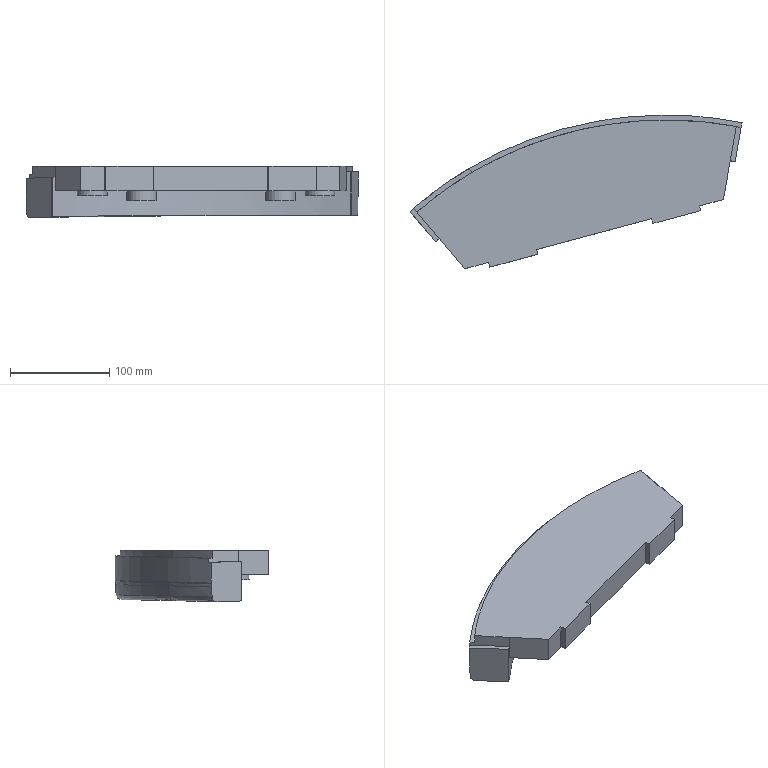Part | NX | features solid 2 | 1 solid | 46 faces | box 335.149 x 155.175 x 52.104 mm | volume 1136931 mm3 | spline 25 | plane 17 | cylinder 4 | commonest cylinder face diameters 30 x4